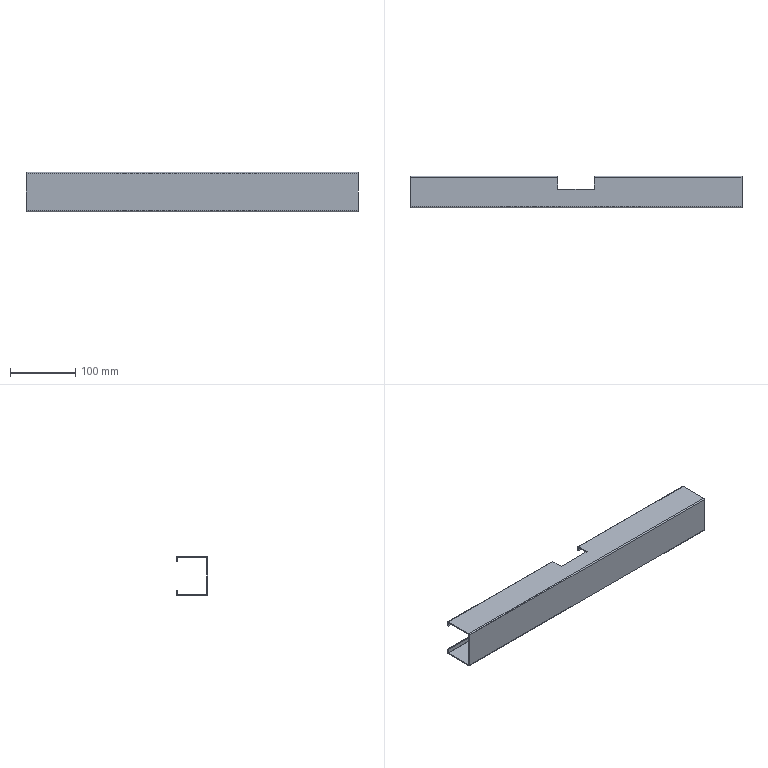Part | 1 solid | 62 faces | box 510 x 48 x 60 mm | volume 121359 mm3 | plane 50 | cylinder 12 | commonest cylinder face diameters 0.4 x6 3.4 x6
STEP:
#1=CARTESIAN_POINT('',(-28.,48.,28.3));
#2=VERTEX_POINT('',#1);
#3=CARTESIAN_POINT('',(-28.,48.,22.));
#4=VERTEX_POINT('',#3);
#5=CARTESIAN_POINT('',(-28.,48.,22.));
#6=DIRECTION('',(0.,0.,-1.));
#7=VECTOR('',#6,1000.);
#8=LINE('',#5,#7);
#9=EDGE_CURVE('',#2,#4,#8,.T.);
#10=ORIENTED_EDGE('',*,*,#9,.F.);
#11=CARTESIAN_POINT('',(-28.,46.5,28.3));
#12=VERTEX_POINT('',#11);
#13=CARTESIAN_POINT('',(-28.,48.,28.3));
#14=DIRECTION('',(0.,-1.,0.));
#15=VECTOR('',#14,1000.);
#16=LINE('',#13,#15);
#17=EDGE_CURVE('',#2,#12,#16,.T.);
#18=ORIENTED_EDGE('',*,*,#17,.T.);
#19=CARTESIAN_POINT('',(-28.,46.5,22.));
#20=VERTEX_POINT('',#19);
#21=CARTESIAN_POINT('',(-28.,46.5,22.));
#22=DIRECTION('',(0.,0.,-1.));
#23=VECTOR('',#22,1000.);
#24=LINE('',#21,#23);
#25=EDGE_CURVE('',#12,#20,#24,.T.);
#26=ORIENTED_EDGE('',*,*,#25,.T.);
#27=CARTESIAN_POINT('',(-28.,48.,22.));
#28=DIRECTION('',(0.,1.,0.));
#29=VECTOR('',#28,1000.);
#30=LINE('',#27,#29);
#31=EDGE_CURVE('',#20,#4,#30,.T.);
#32=ORIENTED_EDGE('',*,*,#31,.T.);
#33=EDGE_LOOP('',(#10,#18,#26,#32));
#34=FACE_OUTER_BOUND('',#33,.T.);
#35=CARTESIAN_POINT('',(-28.,68.,-30.));
#36=DIRECTION('',(-1.,0.,0.));
#37=DIRECTION('',(0.,0.,1.));
#38=AXIS2_PLACEMENT_3D('',#35,#36,#37);
#39=PLANE('',#38);
#40=ADVANCED_FACE('',(#34),#39,.F.);
#41=CARTESIAN_POINT('',(-28.,28.,28.5));
#42=VERTEX_POINT('',#41);
#43=CARTESIAN_POINT('',(-28.,46.3,28.5));
#44=VERTEX_POINT('',#43);
#45=CARTESIAN_POINT('',(-28.,48.,28.5));
#46=DIRECTION('',(0.,1.,0.));
#47=VECTOR('',#46,1000.);
#48=LINE('',#45,#47);
#49=EDGE_CURVE('',#42,#44,#48,.T.);
#50=ORIENTED_EDGE('',*,*,#49,.T.);
#51=CARTESIAN_POINT('',(-28.,46.3,30.));
#52=VERTEX_POINT('',#51);
#53=CARTESIAN_POINT('',(-28.,46.3,28.5));
#54=DIRECTION('',(0.,0.,1.));
#55=VECTOR('',#54,1000.);
#56=LINE('',#53,#55);
#57=EDGE_CURVE('',#44,#52,#56,.T.);
#58=ORIENTED_EDGE('',*,*,#57,.T.);
#59=CARTESIAN_POINT('',(-28.,28.,30.));
#60=VERTEX_POINT('',#59);
#61=CARTESIAN_POINT('',(-28.,48.,30.));
#62=DIRECTION('',(0.,1.,0.));
#63=VECTOR('',#62,1000.);
#64=LINE('',#61,#63);
#65=EDGE_CURVE('',#60,#52,#64,.T.);
#66=ORIENTED_EDGE('',*,*,#65,.F.);
#67=CARTESIAN_POINT('',(-28.,28.,-30.));
#68=DIRECTION('',(0.,0.,1.));
#69=VECTOR('',#68,1000.);
#70=LINE('',#67,#69);
#71=EDGE_CURVE('',#42,#60,#70,.T.);
#72=ORIENTED_EDGE('',*,*,#71,.F.);
#73=EDGE_LOOP('',(#50,#58,#66,#72));
#74=FACE_OUTER_BOUND('',#73,.T.);
#75=CARTESIAN_POINT('',(-28.,68.,-30.));
#76=DIRECTION('',(-1.,0.,0.));
#77=DIRECTION('',(0.,0.,1.));
#78=AXIS2_PLACEMENT_3D('',#75,#76,#77);
#79=PLANE('',#78);
#80=ADVANCED_FACE('',(#74),#79,.F.);
#81=CARTESIAN_POINT('',(28.,46.5,22.));
#82=VERTEX_POINT('',#81);
#83=CARTESIAN_POINT('',(28.,46.5,28.3));
#84=VERTEX_POINT('',#83);
#85=CARTESIAN_POINT('',(28.,46.5,22.));
#86=DIRECTION('',(0.,0.,1.));
#87=VECTOR('',#86,1000.);
#88=LINE('',#85,#87);
#89=EDGE_CURVE('',#82,#84,#88,.T.);
#90=ORIENTED_EDGE('',*,*,#89,.T.);
#91=CARTESIAN_POINT('',(28.,48.,28.3));
#92=VERTEX_POINT('',#91);
#93=CARTESIAN_POINT('',(28.,46.5,28.3));
#94=DIRECTION('',(0.,1.,0.));
#95=VECTOR('',#94,1000.);
#96=LINE('',#93,#95);
#97=EDGE_CURVE('',#84,#92,#96,.T.);
#98=ORIENTED_EDGE('',*,*,#97,.T.);
#99=CARTESIAN_POINT('',(28.,48.,22.));
#100=VERTEX_POINT('',#99);
#101=CARTESIAN_POINT('',(28.,48.,22.));
#102=DIRECTION('',(0.,0.,1.));
#103=VECTOR('',#102,1000.);
#104=LINE('',#101,#103);
#105=EDGE_CURVE('',#100,#92,#104,.T.);
#106=ORIENTED_EDGE('',*,*,#105,.F.);
#107=CARTESIAN_POINT('',(28.,48.,22.));
#108=DIRECTION('',(0.,-1.,0.));
#109=VECTOR('',#108,1000.);
#110=LINE('',#107,#109);
#111=EDGE_CURVE('',#100,#82,#110,.T.);
#112=ORIENTED_EDGE('',*,*,#111,.T.);
#113=EDGE_LOOP('',(#90,#98,#106,#112));
#114=FACE_OUTER_BOUND('',#113,.T.);
#115=CARTESIAN_POINT('',(28.,68.,-30.));
#116=DIRECTION('',(1.,0.,0.));
#117=DIRECTION('',(0.,0.,-1.));
#118=AXIS2_PLACEMENT_3D('',#115,#116,#117);
#119=PLANE('',#118);
#120=ADVANCED_FACE('',(#114),#119,.F.);
#121=CARTESIAN_POINT('',(28.,46.3,30.));
#122=VERTEX_POINT('',#121);
#123=CARTESIAN_POINT('',(28.,28.,30.));
#124=VERTEX_POINT('',#123);
#125=CARTESIAN_POINT('',(28.,48.,30.));
#126=DIRECTION('',(0.,-1.,0.));
#127=VECTOR('',#126,1000.);
#128=LINE('',#125,#127);
#129=EDGE_CURVE('',#122,#124,#128,.T.);
#130=ORIENTED_EDGE('',*,*,#129,.F.);
#131=CARTESIAN_POINT('',(28.,46.3,28.5));
#132=VERTEX_POINT('',#131);
#133=CARTESIAN_POINT('',(28.,46.3,30.));
#134=DIRECTION('',(0.,0.,-1.));
#135=VECTOR('',#134,1000.);
#136=LINE('',#133,#135);
#137=EDGE_CURVE('',#122,#132,#136,.T.);
#138=ORIENTED_EDGE('',*,*,#137,.T.);
#139=CARTESIAN_POINT('',(28.,28.,28.5));
#140=VERTEX_POINT('',#139);
#141=CARTESIAN_POINT('',(28.,48.,28.5));
#142=DIRECTION('',(0.,-1.,0.));
#143=VECTOR('',#142,1000.);
#144=LINE('',#141,#143);
#145=EDGE_CURVE('',#132,#140,#144,.T.);
#146=ORIENTED_EDGE('',*,*,#145,.T.);
#147=CARTESIAN_POINT('',(28.,28.,-30.));
#148=DIRECTION('',(0.,0.,1.));
#149=VECTOR('',#148,1000.);
#150=LINE('',#147,#149);
#151=EDGE_CURVE('',#140,#124,#150,.T.);
#152=ORIENTED_EDGE('',*,*,#151,.T.);
#153=EDGE_LOOP('',(#130,#138,#146,#152));
#154=FACE_OUTER_BOUND('',#153,.T.);
#155=CARTESIAN_POINT('',(28.,68.,-30.));
#156=DIRECTION('',(1.,0.,0.));
#157=DIRECTION('',(0.,0.,-1.));
#158=AXIS2_PLACEMENT_3D('',#155,#156,#157);
#159=PLANE('',#158);
#160=ADVANCED_FACE('',(#154),#159,.F.);
#161=CARTESIAN_POINT('',(-28.,46.5,-22.));
#162=VERTEX_POINT('',#161);
#163=CARTESIAN_POINT('',(-28.,46.5,-28.3));
#164=VERTEX_POINT('',#163);
#165=CARTESIAN_POINT('',(-28.,46.5,-30.));
#166=DIRECTION('',(0.,0.,-1.));
#167=VECTOR('',#166,1000.);
#168=LINE('',#165,#167);
#169=EDGE_CURVE('',#162,#164,#168,.T.);
#170=ORIENTED_EDGE('',*,*,#169,.T.);
#171=CARTESIAN_POINT('',(-28.,48.,-28.3));
#172=VERTEX_POINT('',#171);
#173=CARTESIAN_POINT('',(-28.,46.5,-28.3));
#174=DIRECTION('',(0.,1.,0.));
#175=VECTOR('',#174,1000.);
#176=LINE('',#173,#175);
#177=EDGE_CURVE('',#164,#172,#176,.T.);
#178=ORIENTED_EDGE('',*,*,#177,.T.);
#179=CARTESIAN_POINT('',(-28.,48.,-22.));
#180=VERTEX_POINT('',#179);
#181=CARTESIAN_POINT('',(-28.,48.,-30.));
#182=DIRECTION('',(0.,0.,-1.));
#183=VECTOR('',#182,1000.);
#184=LINE('',#181,#183);
#185=EDGE_CURVE('',#180,#172,#184,.T.);
#186=ORIENTED_EDGE('',*,*,#185,.F.);
#187=CARTESIAN_POINT('',(-28.,46.5,-22.));
#188=DIRECTION('',(0.,-1.,0.));
#189=VECTOR('',#188,1000.);
#190=LINE('',#187,#189);
#191=EDGE_CURVE('',#180,#162,#190,.T.);
#192=ORIENTED_EDGE('',*,*,#191,.T.);
#193=EDGE_LOOP('',(#170,#178,#186,#192));
#194=FACE_OUTER_BOUND('',#193,.T.);
#195=CARTESIAN_POINT('',(-28.,68.,-30.));
#196=DIRECTION('',(-1.,0.,0.));
#197=DIRECTION('',(0.,0.,1.));
#198=AXIS2_PLACEMENT_3D('',#195,#196,#197);
#199=PLANE('',#198);
#200=ADVANCED_FACE('',(#194),#199,.F.);
#201=CARTESIAN_POINT('',(-28.,46.3,-30.));
#202=VERTEX_POINT('',#201);
#203=CARTESIAN_POINT('',(-28.,28.,-30.));
#204=VERTEX_POINT('',#203);
#205=CARTESIAN_POINT('',(-28.,68.,-30.));
#206=DIRECTION('',(0.,-1.,0.));
#207=VECTOR('',#206,1000.);
#208=LINE('',#205,#207);
#209=EDGE_CURVE('',#202,#204,#208,.T.);
#210=ORIENTED_EDGE('',*,*,#209,.F.);
#211=CARTESIAN_POINT('',(-28.,46.3,-28.5));
#212=VERTEX_POINT('',#211);
#213=CARTESIAN_POINT('',(-28.,46.3,-30.));
#214=DIRECTION('',(0.,0.,1.));
#215=VECTOR('',#214,1000.);
#216=LINE('',#213,#215);
#217=EDGE_CURVE('',#202,#212,#216,.T.);
#218=ORIENTED_EDGE('',*,*,#217,.T.);
#219=CARTESIAN_POINT('',(-28.,28.,-28.5));
#220=VERTEX_POINT('',#219);
#221=CARTESIAN_POINT('',(-28.,0.,-28.5));
#222=DIRECTION('',(0.,-1.,0.));
#223=VECTOR('',#222,1000.);
#224=LINE('',#221,#223);
#225=EDGE_CURVE('',#212,#220,#224,.T.);
#226=ORIENTED_EDGE('',*,*,#225,.T.);
#227=CARTESIAN_POINT('',(-28.,28.,-30.));
#228=DIRECTION('',(0.,0.,1.));
#229=VECTOR('',#228,1000.);
#230=LINE('',#227,#229);
#231=EDGE_CURVE('',#204,#220,#230,.T.);
#232=ORIENTED_EDGE('',*,*,#231,.F.);
#233=EDGE_LOOP('',(#210,#218,#226,#232));
#234=FACE_OUTER_BOUND('',#233,.T.);
#235=CARTESIAN_POINT('',(-28.,68.,-30.));
#236=DIRECTION('',(-1.,0.,0.));
#237=DIRECTION('',(0.,0.,1.));
#238=AXIS2_PLACEMENT_3D('',#235,#236,#237);
#239=PLANE('',#238);
#240=ADVANCED_FACE('',(#234),#239,.F.);
#241=CARTESIAN_POINT('',(28.,48.,-28.3));
#242=VERTEX_POINT('',#241);
#243=CARTESIAN_POINT('',(28.,48.,-22.));
#244=VERTEX_POINT('',#243);
#245=CARTESIAN_POINT('',(28.,48.,-30.));
#246=DIRECTION('',(0.,0.,1.));
#247=VECTOR('',#246,1000.);
#248=LINE('',#245,#247);
#249=EDGE_CURVE('',#242,#244,#248,.T.);
#250=ORIENTED_EDGE('',*,*,#249,.F.);
#251=CARTESIAN_POINT('',(28.,46.5,-28.3));
#252=VERTEX_POINT('',#251);
#253=CARTESIAN_POINT('',(28.,48.,-28.3));
#254=DIRECTION('',(0.,-1.,0.));
#255=VECTOR('',#254,1000.);
#256=LINE('',#253,#255);
#257=EDGE_CURVE('',#242,#252,#256,.T.);
#258=ORIENTED_EDGE('',*,*,#257,.T.);
#259=CARTESIAN_POINT('',(28.,46.5,-22.));
#260=VERTEX_POINT('',#259);
#261=CARTESIAN_POINT('',(28.,46.5,-30.));
#262=DIRECTION('',(0.,0.,1.));
#263=VECTOR('',#262,1000.);
#264=LINE('',#261,#263);
#265=EDGE_CURVE('',#252,#260,#264,.T.);
#266=ORIENTED_EDGE('',*,*,#265,.T.);
#267=CARTESIAN_POINT('',(28.,46.5,-22.));
#268=DIRECTION('',(0.,1.,0.));
#269=VECTOR('',#268,1000.);
#270=LINE('',#267,#269);
#271=EDGE_CURVE('',#260,#244,#270,.T.);
#272=ORIENTED_EDGE('',*,*,#271,.T.);
#273=EDGE_LOOP('',(#250,#258,#266,#272));
#274=FACE_OUTER_BOUND('',#273,.T.);
#275=CARTESIAN_POINT('',(28.,68.,-30.));
#276=DIRECTION('',(1.,0.,0.));
#277=DIRECTION('',(0.,0.,-1.));
#278=AXIS2_PLACEMENT_3D('',#275,#276,#277);
#279=PLANE('',#278);
#280=ADVANCED_FACE('',(#274),#279,.F.);
#281=CARTESIAN_POINT('',(28.,28.,-28.5));
#282=VERTEX_POINT('',#281);
#283=CARTESIAN_POINT('',(28.,46.3,-28.5));
#284=VERTEX_POINT('',#283);
#285=CARTESIAN_POINT('',(28.,0.,-28.5));
#286=DIRECTION('',(0.,1.,0.));
#287=VECTOR('',#286,1000.);
#288=LINE('',#285,#287);
#289=EDGE_CURVE('',#282,#284,#288,.T.);
#290=ORIENTED_EDGE('',*,*,#289,.T.);
#291=CARTESIAN_POINT('',(28.,46.3,-30.));
#292=VERTEX_POINT('',#291);
#293=CARTESIAN_POINT('',(28.,46.3,-28.5));
#294=DIRECTION('',(0.,0.,-1.));
#295=VECTOR('',#294,1000.);
#296=LINE('',#293,#295);
#297=EDGE_CURVE('',#284,#292,#296,.T.);
#298=ORIENTED_EDGE('',*,*,#297,.T.);
#299=CARTESIAN_POINT('',(28.,28.,-30.));
#300=VERTEX_POINT('',#299);
#301=CARTESIAN_POINT('',(28.,68.,-30.));
#302=DIRECTION('',(0.,1.,0.));
#303=VECTOR('',#302,1000.);
#304=LINE('',#301,#303);
#305=EDGE_CURVE('',#300,#292,#304,.T.);
#306=ORIENTED_EDGE('',*,*,#305,.F.);
#307=CARTESIAN_POINT('',(28.,28.,-30.));
#308=DIRECTION('',(0.,0.,1.));
#309=VECTOR('',#308,1000.);
#310=LINE('',#307,#309);
#311=EDGE_CURVE('',#300,#282,#310,.T.);
#312=ORIENTED_EDGE('',*,*,#311,.T.);
#313=EDGE_LOOP('',(#290,#298,#306,#312));
#314=FACE_OUTER_BOUND('',#313,.T.);
#315=CARTESIAN_POINT('',(28.,68.,-30.));
#316=DIRECTION('',(1.,0.,0.));
#317=DIRECTION('',(0.,0.,-1.));
#318=AXIS2_PLACEMENT_3D('',#315,#316,#317);
#319=PLANE('',#318);
#320=ADVANCED_FACE('',(#314),#319,.F.);
#321=CARTESIAN_POINT('',(255.,48.,-28.3));
#322=VERTEX_POINT('',#321);
#323=CARTESIAN_POINT('',(255.,48.,-28.3));
#324=DIRECTION('',(-1.,0.,0.));
#325=VECTOR('',#324,1000.);
#326=LINE('',#323,#325);
#327=EDGE_CURVE('',#322,#242,#326,.T.);
#328=ORIENTED_EDGE('',*,*,#327,.T.);
#329=ORIENTED_EDGE('',*,*,#249,.T.);
#330=CARTESIAN_POINT('',(255.,48.,-22.));
#331=VERTEX_POINT('',#330);
#332=CARTESIAN_POINT('',(255.,48.,-22.));
#333=DIRECTION('',(-1.,0.,0.));
#334=VECTOR('',#333,1000.);
#335=LINE('',#332,#334);
#336=EDGE_CURVE('',#331,#244,#335,.T.);
#337=ORIENTED_EDGE('',*,*,#336,.F.);
#338=CARTESIAN_POINT('',(255.,48.,-30.));
#339=DIRECTION('',(0.,0.,1.));
#340=VECTOR('',#339,1000.);
#341=LINE('',#338,#340);
#342=EDGE_CURVE('',#322,#331,#341,.T.);
#343=ORIENTED_EDGE('',*,*,#342,.F.);
#344=EDGE_LOOP('',(#328,#329,#337,#343));
#345=FACE_OUTER_BOUND('',#344,.T.);
#346=CARTESIAN_POINT('',(255.,48.,-30.));
#347=DIRECTION('',(0.,-1.,0.));
#348=DIRECTION('',(0.,0.,-1.));
#349=AXIS2_PLACEMENT_3D('',#346,#347,#348);
#350=PLANE('',#349);
#351=ADVANCED_FACE('',(#345),#350,.F.);
#352=ORIENTED_EDGE('',*,*,#271,.F.);
#353=CARTESIAN_POINT('',(255.,46.5,-22.));
#354=VERTEX_POINT('',#353);
#355=CARTESIAN_POINT('',(255.,46.5,-22.));
#356=DIRECTION('',(-1.,0.,0.));
#357=VECTOR('',#356,1000.);
#358=LINE('',#355,#357);
#359=EDGE_CURVE('',#354,#260,#358,.T.);
#360=ORIENTED_EDGE('',*,*,#359,.F.);
#361=CARTESIAN_POINT('',(255.,46.5,-22.));
#362=DIRECTION('',(0.,1.,0.));
#363=VECTOR('',#362,1000.);
#364=LINE('',#361,#363);
#365=EDGE_CURVE('',#354,#331,#364,.T.);
#366=ORIENTED_EDGE('',*,*,#365,.T.);
#367=ORIENTED_EDGE('',*,*,#336,.T.);
#368=EDGE_LOOP('',(#352,#360,#366,#367));
#369=FACE_OUTER_BOUND('',#368,.T.);
#370=CARTESIAN_POINT('',(255.,46.5,-22.));
#371=DIRECTION('',(0.,0.,1.));
#372=DIRECTION('',(1.,0.,0.));
#373=AXIS2_PLACEMENT_3D('',#370,#371,#372);
#374=PLANE('',#373);
#375=ADVANCED_FACE('',(#369),#374,.T.);
#376=ORIENTED_EDGE('',*,*,#265,.F.);
#377=CARTESIAN_POINT('',(255.,46.5,-28.3));
#378=VERTEX_POINT('',#377);
#379=CARTESIAN_POINT('',(255.,46.5,-28.3));
#380=DIRECTION('',(-1.,0.,0.));
#381=VECTOR('',#380,1000.);
#382=LINE('',#379,#381);
#383=EDGE_CURVE('',#378,#252,#382,.T.);
#384=ORIENTED_EDGE('',*,*,#383,.F.);
#385=CARTESIAN_POINT('',(255.,46.5,-30.));
#386=DIRECTION('',(0.,0.,1.));
#387=VECTOR('',#386,1000.);
#388=LINE('',#385,#387);
#389=EDGE_CURVE('',#378,#354,#388,.T.);
#390=ORIENTED_EDGE('',*,*,#389,.T.);
#391=ORIENTED_EDGE('',*,*,#359,.T.);
#392=EDGE_LOOP('',(#376,#384,#390,#391));
#393=FACE_OUTER_BOUND('',#392,.T.);
#394=CARTESIAN_POINT('',(255.,46.5,-30.));
#395=DIRECTION('',(0.,-1.,0.));
#396=DIRECTION('',(0.,0.,-1.));
#397=AXIS2_PLACEMENT_3D('',#394,#395,#396);
#398=PLANE('',#397);
#399=ADVANCED_FACE('',(#393),#398,.T.);
#400=CARTESIAN_POINT('',(28.,46.3,-28.3));
#401=DIRECTION('',(1.,0.,0.));
#402=DIRECTION('',(0.,0.,-1.));
#403=AXIS2_PLACEMENT_3D('',#400,#401,#402);
#404=CIRCLE('',#403,0.2);
#405=EDGE_CURVE('',#284,#252,#404,.T.);
#406=ORIENTED_EDGE('',*,*,#405,.F.);
#407=CARTESIAN_POINT('',(255.,46.3,-28.5));
#408=VERTEX_POINT('',#407);
#409=CARTESIAN_POINT('',(255.,46.3,-28.5));
#410=DIRECTION('',(-1.,0.,0.));
#411=VECTOR('',#410,1000.);
#412=LINE('',#409,#411);
#413=EDGE_CURVE('',#408,#284,#412,.T.);
#414=ORIENTED_EDGE('',*,*,#413,.F.);
#415=CARTESIAN_POINT('',(255.,46.3,-28.3));
#416=DIRECTION('',(1.,0.,0.));
#417=DIRECTION('',(0.,0.,-1.));
#418=AXIS2_PLACEMENT_3D('',#415,#416,#417);
#419=CIRCLE('',#418,0.2);
#420=EDGE_CURVE('',#408,#378,#419,.T.);
#421=ORIENTED_EDGE('',*,*,#420,.T.);
#422=ORIENTED_EDGE('',*,*,#383,.T.);
#423=EDGE_LOOP('',(#406,#414,#421,#422));
#424=FACE_OUTER_BOUND('',#423,.T.);
#425=CARTESIAN_POINT('',(255.,46.3,-28.3));
#426=DIRECTION('',(-1.,0.,0.));
#427=DIRECTION('',(0.,0.,1.));
#428=AXIS2_PLACEMENT_3D('',#425,#426,#427);
#429=CYLINDRICAL_SURFACE('',#428,0.2);
#430=ADVANCED_FACE('',(#424),#429,.F.);
#431=CARTESIAN_POINT('',(28.,46.3,28.3));
#432=DIRECTION('',(1.,0.,0.));
#433=DIRECTION('',(0.,0.,-1.));
#434=AXIS2_PLACEMENT_3D('',#431,#432,#433);
#435=CIRCLE('',#434,0.2);
#436=EDGE_CURVE('',#84,#132,#435,.T.);
#437=ORIENTED_EDGE('',*,*,#436,.F.);
#438=CARTESIAN_POINT('',(255.,46.5,28.3));
#439=VERTEX_POINT('',#438);
#440=CARTESIAN_POINT('',(255.,46.5,28.3));
#441=DIRECTION('',(-1.,0.,0.));
#442=VECTOR('',#441,1000.);
#443=LINE('',#440,#442);
#444=EDGE_CURVE('',#439,#84,#443,.T.);
#445=ORIENTED_EDGE('',*,*,#444,.F.);
#446=CARTESIAN_POINT('',(255.,46.3,28.5));
#447=VERTEX_POINT('',#446);
#448=CARTESIAN_POINT('',(255.,46.3,28.3));
#449=DIRECTION('',(1.,0.,0.));
#450=DIRECTION('',(0.,0.,-1.));
#451=AXIS2_PLACEMENT_3D('',#448,#449,#450);
#452=CIRCLE('',#451,0.2);
#453=EDGE_CURVE('',#439,#447,#452,.T.);
#454=ORIENTED_EDGE('',*,*,#453,.T.);
#455=CARTESIAN_POINT('',(255.,46.3,28.5));
#456=DIRECTION('',(-1.,0.,0.));
#457=VECTOR('',#456,1000.);
#458=LINE('',#455,#457);
#459=EDGE_CURVE('',#447,#132,#458,.T.);
#460=ORIENTED_EDGE('',*,*,#459,.T.);
#461=EDGE_LOOP('',(#437,#445,#454,#460));
#462=FACE_OUTER_BOUND('',#461,.T.);
#463=CARTESIAN_POINT('',(255.,46.3,28.3));
#464=DIRECTION('',(-1.,0.,0.));
#465=DIRECTION('',(0.,0.,1.));
#466=AXIS2_PLACEMENT_3D('',#463,#464,#465);
#467=CYLINDRICAL_SURFACE('',#466,0.2);
#468=ADVANCED_FACE('',(#462),#467,.F.);
#469=ORIENTED_EDGE('',*,*,#89,.F.);
#470=CARTESIAN_POINT('',(255.,46.5,22.));
#471=VERTEX_POINT('',#470);
#472=CARTESIAN_POINT('',(255.,46.5,22.));
#473=DIRECTION('',(-1.,0.,0.));
#474=VECTOR('',#473,1000.);
#475=LINE('',#472,#474);
#476=EDGE_CURVE('',#471,#82,#475,.T.);
#477=ORIENTED_EDGE('',*,*,#476,.F.);
#478=CARTESIAN_POINT('',(255.,46.5,22.));
#479=DIRECTION('',(0.,0.,1.));
#480=VECTOR('',#479,1000.);
#481=LINE('',#478,#480);
#482=EDGE_CURVE('',#471,#439,#481,.T.);
#483=ORIENTED_EDGE('',*,*,#482,.T.);
#484=ORIENTED_EDGE('',*,*,#444,.T.);
#485=EDGE_LOOP('',(#469,#477,#483,#484));
#486=FACE_OUTER_BOUND('',#485,.T.);
#487=CARTESIAN_POINT('',(255.,46.5,22.));
#488=DIRECTION('',(0.,-1.,0.));
#489=DIRECTION('',(0.,0.,-1.));
#490=AXIS2_PLACEMENT_3D('',#487,#488,#489);
#491=PLANE('',#490);
#492=ADVANCED_FACE('',(#486),#491,.T.);
#493=ORIENTED_EDGE('',*,*,#111,.F.);
#494=CARTESIAN_POINT('',(255.,48.,22.));
#495=VERTEX_POINT('',#494);
#496=CARTESIAN_POINT('',(255.,48.,22.));
#497=DIRECTION('',(-1.,0.,0.));
#498=VECTOR('',#497,1000.);
#499=LINE('',#496,#498);
#500=EDGE_CURVE('',#495,#100,#499,.T.);
#501=ORIENTED_EDGE('',*,*,#500,.F.);
#502=CARTESIAN_POINT('',(255.,48.,22.));
#503=DIRECTION('',(0.,-1.,0.));
#504=VECTOR('',#503,1000.);
#505=LINE('',#502,#504);
#506=EDGE_CURVE('',#495,#471,#505,.T.);
#507=ORIENTED_EDGE('',*,*,#506,.T.);
#508=ORIENTED_EDGE('',*,*,#476,.T.);
#509=EDGE_LOOP('',(#493,#501,#507,#508));
#510=FACE_OUTER_BOUND('',#509,.T.);
#511=CARTESIAN_POINT('',(255.,48.,22.));
#512=DIRECTION('',(0.,0.,-1.));
#513=DIRECTION('',(-1.,0.,0.));
#514=AXIS2_PLACEMENT_3D('',#511,#512,#513);
#515=PLANE('',#514);
#516=ADVANCED_FACE('',(#510),#515,.T.);
#517=ORIENTED_EDGE('',*,*,#500,.T.);
#518=ORIENTED_EDGE('',*,*,#105,.T.);
#519=CARTESIAN_POINT('',(255.,48.,28.3));
#520=VERTEX_POINT('',#519);
#521=CARTESIAN_POINT('',(255.,48.,28.3));
#522=DIRECTION('',(-1.,0.,0.));
#523=VECTOR('',#522,1000.);
#524=LINE('',#521,#523);
#525=EDGE_CURVE('',#520,#92,#524,.T.);
#526=ORIENTED_EDGE('',*,*,#525,.F.);
#527=CARTESIAN_POINT('',(255.,48.,22.));
#528=DIRECTION('',(0.,0.,1.));
#529=VECTOR('',#528,1000.);
#530=LINE('',#527,#529);
#531=EDGE_CURVE('',#495,#520,#530,.T.);
#532=ORIENTED_EDGE('',*,*,#531,.F.);
#533=EDGE_LOOP('',(#517,#518,#526,#532));
#534=FACE_OUTER_BOUND('',#533,.T.);
#535=CARTESIAN_POINT('',(255.,48.,22.));
#536=DIRECTION('',(0.,-1.,0.));
#537=DIRECTION('',(0.,0.,-1.));
#538=AXIS2_PLACEMENT_3D('',#535,#536,#537);
#539=PLANE('',#538);
#540=ADVANCED_FACE('',(#534),#539,.F.);
#541=ORIENTED_EDGE('',*,*,#525,.T.);
#542=CARTESIAN_POINT('',(28.,46.3,28.3));
#543=DIRECTION('',(1.,0.,0.));
#544=DIRECTION('',(0.,0.,-1.));
#545=AXIS2_PLACEMENT_3D('',#542,#543,#544);
#546=CIRCLE('',#545,1.7);
#547=EDGE_CURVE('',#92,#122,#546,.T.);
#548=ORIENTED_EDGE('',*,*,#547,.T.);
#549=CARTESIAN_POINT('',(255.,46.3,30.));
#550=VERTEX_POINT('',#549);
#551=CARTESIAN_POINT('',(255.,46.3,30.));
#552=DIRECTION('',(-1.,0.,0.));
#553=VECTOR('',#552,1000.);
#554=LINE('',#551,#553);
#555=EDGE_CURVE('',#550,#122,#554,.T.);
#556=ORIENTED_EDGE('',*,*,#555,.F.);
#557=CARTESIAN_POINT('',(255.,46.3,28.3));
#558=DIRECTION('',(1.,0.,0.));
#559=DIRECTION('',(0.,0.,1.));
#560=AXIS2_PLACEMENT_3D('',#557,#558,#559);
#561=CIRCLE('',#560,1.7);
#562=EDGE_CURVE('',#520,#550,#561,.T.);
#563=ORIENTED_EDGE('',*,*,#562,.F.);
#564=EDGE_LOOP('',(#541,#548,#556,#563));
#565=FACE_OUTER_BOUND('',#564,.T.);
#566=CARTESIAN_POINT('',(255.,46.3,28.3));
#567=DIRECTION('',(-1.,0.,0.));
#568=DIRECTION('',(0.,0.,1.));
#569=AXIS2_PLACEMENT_3D('',#566,#567,#568);
#570=CYLINDRICAL_SURFACE('',#569,1.7);
#571=ADVANCED_FACE('',(#565),#570,.T.);
#572=CARTESIAN_POINT('',(255.,46.3,-30.));
#573=VERTEX_POINT('',#572);
#574=CARTESIAN_POINT('',(255.,46.3,-30.));
#575=DIRECTION('',(-1.,0.,0.));
#576=VECTOR('',#575,1000.);
#577=LINE('',#574,#576);
#578=EDGE_CURVE('',#573,#292,#577,.T.);
#579=ORIENTED_EDGE('',*,*,#578,.T.);
#580=CARTESIAN_POINT('',(28.,46.3,-28.3));
#581=DIRECTION('',(1.,0.,0.));
#582=DIRECTION('',(0.,0.,-1.));
#583=AXIS2_PLACEMENT_3D('',#580,#581,#582);
#584=CIRCLE('',#583,1.7);
#585=EDGE_CURVE('',#292,#242,#584,.T.);
#586=ORIENTED_EDGE('',*,*,#585,.T.);
#587=ORIENTED_EDGE('',*,*,#327,.F.);
#588=CARTESIAN_POINT('',(255.,46.3,-28.3));
#589=DIRECTION('',(1.,0.,0.));
#590=DIRECTION('',(0.,0.,1.));
#591=AXIS2_PLACEMENT_3D('',#588,#589,#590);
#592=CIRCLE('',#591,1.7);
#593=EDGE_CURVE('',#573,#322,#592,.T.);
#594=ORIENTED_EDGE('',*,*,#593,.F.);
#595=EDGE_LOOP('',(#579,#586,#587,#594));
#596=FACE_OUTER_BOUND('',#595,.T.);
#597=CARTESIAN_POINT('',(255.,46.3,-28.3));
#598=DIRECTION('',(-1.,0.,0.));
#599=DIRECTION('',(0.,0.,1.));
#600=AXIS2_PLACEMENT_3D('',#597,#598,#599);
#601=CYLINDRICAL_SURFACE('',#600,1.7);
#602=ADVANCED_FACE('',(#596),#601,.T.);
#603=CARTESIAN_POINT('',(255.,48.,28.3));
#604=DIRECTION('',(0.,-1.,0.));
#605=VECTOR('',#604,1000.);
#606=LINE('',#603,#605);
#607=EDGE_CURVE('',#520,#439,#606,.T.);
#608=ORIENTED_EDGE('',*,*,#607,.F.);
#609=ORIENTED_EDGE('',*,*,#562,.T.);
#610=CARTESIAN_POINT('',(255.,46.3,28.5));
#611=DIRECTION('',(0.,0.,1.));
#612=VECTOR('',#611,1000.);
#613=LINE('',#610,#612);
#614=EDGE_CURVE('',#447,#550,#613,.T.);
#615=ORIENTED_EDGE('',*,*,#614,.F.);
#616=ORIENTED_EDGE('',*,*,#453,.F.);
#617=EDGE_LOOP('',(#608,#609,#615,#616));
#618=FACE_OUTER_BOUND('',#617,.T.);
#619=CARTESIAN_POINT('',(255.,48.,28.3));
#620=DIRECTION('',(1.,0.,0.));
#621=DIRECTION('',(0.,0.,-1.));
#622=AXIS2_PLACEMENT_3D('',#619,#620,#621);
#623=PLANE('',#622);
#624=ADVANCED_FACE('',(#618),#623,.T.);
#625=ORIENTED_EDGE('',*,*,#531,.T.);
#626=ORIENTED_EDGE('',*,*,#607,.T.);
#627=ORIENTED_EDGE('',*,*,#482,.F.);
#628=ORIENTED_EDGE('',*,*,#506,.F.);
#629=EDGE_LOOP('',(#625,#626,#627,#628));
#630=FACE_OUTER_BOUND('',#629,.T.);
#631=CARTESIAN_POINT('',(255.,46.3,28.5));
#632=DIRECTION('',(1.,0.,0.));
#633=DIRECTION('',(0.,0.,-1.));
#634=AXIS2_PLACEMENT_3D('',#631,#632,#633);
#635=PLANE('',#634);
#636=ADVANCED_FACE('',(#630),#635,.T.);
#637=CARTESIAN_POINT('',(-255.,46.3,30.));
#638=VERTEX_POINT('',#637);
#639=CARTESIAN_POINT('',(-255.,46.3,28.5));
#640=VERTEX_POINT('',#639);
#641=CARTESIAN_POINT('',(-255.,46.3,30.));
#642=DIRECTION('',(0.,0.,-1.));
#643=VECTOR('',#642,1000.);
#644=LINE('',#641,#643);
#645=EDGE_CURVE('',#638,#640,#644,.T.);
#646=ORIENTED_EDGE('',*,*,#645,.F.);
#647=CARTESIAN_POINT('',(-255.,48.,28.3));
#648=VERTEX_POINT('',#647);
#649=CARTESIAN_POINT('',(-255.,46.3,28.3));
#650=DIRECTION('',(1.,0.,0.));
#651=DIRECTION('',(0.,0.,1.));
#652=AXIS2_PLACEMENT_3D('',#649,#650,#651);
#653=CIRCLE('',#652,1.7);
#654=EDGE_CURVE('',#648,#638,#653,.T.);
#655=ORIENTED_EDGE('',*,*,#654,.F.);
#656=CARTESIAN_POINT('',(-255.,46.5,28.3));
#657=VERTEX_POINT('',#656);
#658=CARTESIAN_POINT('',(-255.,46.5,28.3));
#659=DIRECTION('',(0.,1.,0.));
#660=VECTOR('',#659,1000.);
#661=LINE('',#658,#660);
#662=EDGE_CURVE('',#657,#648,#661,.T.);
#663=ORIENTED_EDGE('',*,*,#662,.F.);
#664=CARTESIAN_POINT('',(-255.,46.3,28.3));
#665=DIRECTION('',(1.,0.,0.));
#666=DIRECTION('',(0.,0.,-1.));
#667=AXIS2_PLACEMENT_3D('',#664,#665,#666);
#668=CIRCLE('',#667,0.2);
#669=EDGE_CURVE('',#657,#640,#668,.T.);
#670=ORIENTED_EDGE('',*,*,#669,.T.);
#671=EDGE_LOOP('',(#646,#655,#663,#670));
#672=FACE_OUTER_BOUND('',#671,.T.);
#673=CARTESIAN_POINT('',(-255.,46.3,30.));
#674=DIRECTION('',(-1.,0.,0.));
#675=DIRECTION('',(0.,0.,1.));
#676=AXIS2_PLACEMENT_3D('',#673,#674,#675);
#677=PLANE('',#676);
#678=ADVANCED_FACE('',(#672),#677,.T.);
#679=CARTESIAN_POINT('',(-255.,1.7,30.));
#680=VERTEX_POINT('',#679);
#681=CARTESIAN_POINT('',(-255.,48.,30.));
#682=DIRECTION('',(0.,-1.,0.));
#683=VECTOR('',#682,1000.);
#684=LINE('',#681,#683);
#685=EDGE_CURVE('',#638,#680,#684,.T.);
#686=ORIENTED_EDGE('',*,*,#685,.F.);
#687=ORIENTED_EDGE('',*,*,#645,.T.);
#688=CARTESIAN_POINT('',(-255.,1.7,28.5));
#689=VERTEX_POINT('',#688);
#690=CARTESIAN_POINT('',(-255.,48.,28.5));
#691=DIRECTION('',(0.,-1.,0.));
#692=VECTOR('',#691,1000.);
#693=LINE('',#690,#692);
#694=EDGE_CURVE('',#640,#689,#693,.T.);
#695=ORIENTED_EDGE('',*,*,#694,.T.);
#696=CARTESIAN_POINT('',(-255.,1.7,28.5));
#697=DIRECTION('',(0.,0.,1.));
#698=VECTOR('',#697,1000.);
#699=LINE('',#696,#698);
#700=EDGE_CURVE('',#689,#680,#699,.T.);
#701=ORIENTED_EDGE('',*,*,#700,.T.);
#702=EDGE_LOOP('',(#686,#687,#695,#701));
#703=FACE_OUTER_BOUND('',#702,.T.);
#704=CARTESIAN_POINT('',(-255.,46.5,28.3));
#705=DIRECTION('',(-1.,0.,0.));
#706=DIRECTION('',(0.,0.,1.));
#707=AXIS2_PLACEMENT_3D('',#704,#705,#706);
#708=PLANE('',#707);
#709=ADVANCED_FACE('',(#703),#708,.T.);
#710=CARTESIAN_POINT('',(255.,1.7,30.));
#711=VERTEX_POINT('',#710);
#712=CARTESIAN_POINT('',(255.,1.7,28.5));
#713=VERTEX_POINT('',#712);
#714=CARTESIAN_POINT('',(255.,1.7,30.));
#715=DIRECTION('',(0.,0.,-1.));
#716=VECTOR('',#715,1000.);
#717=LINE('',#714,#716);
#718=EDGE_CURVE('',#711,#713,#717,.T.);
#719=ORIENTED_EDGE('',*,*,#718,.F.);
#720=CARTESIAN_POINT('',(255.,0.,28.3));
#721=VERTEX_POINT('',#720);
#722=CARTESIAN_POINT('',(255.,1.7,28.3));
#723=DIRECTION('',(1.,0.,0.));
#724=DIRECTION('',(0.,0.,1.));
#725=AXIS2_PLACEMENT_3D('',#722,#723,#724);
#726=CIRCLE('',#725,1.7);
#727=EDGE_CURVE('',#711,#721,#726,.T.);
#728=ORIENTED_EDGE('',*,*,#727,.T.);
#729=CARTESIAN_POINT('',(255.,1.5,28.3));
#730=VERTEX_POINT('',#729);
#731=CARTESIAN_POINT('',(255.,1.5,28.3));
#732=DIRECTION('',(0.,-1.,0.));
#733=VECTOR('',#732,1000.);
#734=LINE('',#731,#733);
#735=EDGE_CURVE('',#730,#721,#734,.T.);
#736=ORIENTED_EDGE('',*,*,#735,.F.);
#737=CARTESIAN_POINT('',(255.,1.7,28.3));
#738=DIRECTION('',(1.,0.,0.));
#739=DIRECTION('',(0.,0.,-1.));
#740=AXIS2_PLACEMENT_3D('',#737,#738,#739);
#741=CIRCLE('',#740,0.2);
#742=EDGE_CURVE('',#713,#730,#741,.T.);
#743=ORIENTED_EDGE('',*,*,#742,.F.);
#744=EDGE_LOOP('',(#719,#728,#736,#743));
#745=FACE_OUTER_BOUND('',#744,.T.);
#746=CARTESIAN_POINT('',(255.,1.7,30.));
#747=DIRECTION('',(1.,0.,0.));
#748=DIRECTION('',(0.,0.,-1.));
#749=AXIS2_PLACEMENT_3D('',#746,#747,#748);
#750=PLANE('',#749);
#751=ADVANCED_FACE('',(#745),#750,.T.);
#752=CARTESIAN_POINT('',(255.,48.,30.));
#753=DIRECTION('',(0.,-1.,0.));
#754=VECTOR('',#753,1000.);
#755=LINE('',#752,#754);
#756=EDGE_CURVE('',#550,#711,#755,.T.);
#757=ORIENTED_EDGE('',*,*,#756,.T.);
#758=ORIENTED_EDGE('',*,*,#718,.T.);
#759=CARTESIAN_POINT('',(255.,48.,28.5));
#760=DIRECTION('',(0.,-1.,0.));
#761=VECTOR('',#760,1000.);
#762=LINE('',#759,#761);
#763=EDGE_CURVE('',#447,#713,#762,.T.);
#764=ORIENTED_EDGE('',*,*,#763,.F.);
#765=ORIENTED_EDGE('',*,*,#614,.T.);
#766=EDGE_LOOP('',(#757,#758,#764,#765));
#767=FACE_OUTER_BOUND('',#766,.T.);
#768=CARTESIAN_POINT('',(255.,1.5,28.3));
#769=DIRECTION('',(1.,0.,0.));
#770=DIRECTION('',(0.,0.,-1.));
#771=AXIS2_PLACEMENT_3D('',#768,#769,#770);
#772=PLANE('',#771);
#773=ADVANCED_FACE('',(#767),#772,.T.);
#774=CARTESIAN_POINT('',(-255.,0.,28.3));
#775=VERTEX_POINT('',#774);
#776=CARTESIAN_POINT('',(-255.,1.5,28.3));
#777=VERTEX_POINT('',#776);
#778=CARTESIAN_POINT('',(-255.,0.,28.3));
#779=DIRECTION('',(0.,1.,0.));
#780=VECTOR('',#779,1000.);
#781=LINE('',#778,#780);
#782=EDGE_CURVE('',#775,#777,#781,.T.);
#783=ORIENTED_EDGE('',*,*,#782,.F.);
#784=CARTESIAN_POINT('',(-255.,1.7,28.3));
#785=DIRECTION('',(1.,0.,0.));
#786=DIRECTION('',(0.,0.,1.));
#787=AXIS2_PLACEMENT_3D('',#784,#785,#786);
#788=CIRCLE('',#787,1.7);
#789=EDGE_CURVE('',#680,#775,#788,.T.);
#790=ORIENTED_EDGE('',*,*,#789,.F.);
#791=ORIENTED_EDGE('',*,*,#700,.F.);
#792=CARTESIAN_POINT('',(-255.,1.7,28.3));
#793=DIRECTION('',(1.,0.,0.));
#794=DIRECTION('',(0.,0.,-1.));
#795=AXIS2_PLACEMENT_3D('',#792,#793,#794);
#796=CIRCLE('',#795,0.2);
#797=EDGE_CURVE('',#689,#777,#796,.T.);
#798=ORIENTED_EDGE('',*,*,#797,.T.);
#799=EDGE_LOOP('',(#783,#790,#791,#798));
#800=FACE_OUTER_BOUND('',#799,.T.);
#801=CARTESIAN_POINT('',(-255.,0.,28.3));
#802=DIRECTION('',(-1.,0.,0.));
#803=DIRECTION('',(0.,0.,1.));
#804=AXIS2_PLACEMENT_3D('',#801,#802,#803);
#805=PLANE('',#804);
#806=ADVANCED_FACE('',(#800),#805,.T.);
#807=CARTESIAN_POINT('',(-255.,0.,-28.3));
#808=VERTEX_POINT('',#807);
#809=CARTESIAN_POINT('',(-255.,0.,30.));
#810=DIRECTION('',(0.,0.,-1.));
#811=VECTOR('',#810,1000.);
#812=LINE('',#809,#811);
#813=EDGE_CURVE('',#775,#808,#812,.T.);
#814=ORIENTED_EDGE('',*,*,#813,.F.);
#815=ORIENTED_EDGE('',*,*,#782,.T.);
#816=CARTESIAN_POINT('',(-255.,1.5,-28.3));
#817=VERTEX_POINT('',#816);
#818=CARTESIAN_POINT('',(-255.,1.5,30.));
#819=DIRECTION('',(0.,0.,-1.));
#820=VECTOR('',#819,1000.);
#821=LINE('',#818,#820);
#822=EDGE_CURVE('',#777,#817,#821,.T.);
#823=ORIENTED_EDGE('',*,*,#822,.T.);
#824=CARTESIAN_POINT('',(-255.,1.5,-28.3));
#825=DIRECTION('',(0.,-1.,0.));
#826=VECTOR('',#825,1000.);
#827=LINE('',#824,#826);
#828=EDGE_CURVE('',#817,#808,#827,.T.);
#829=ORIENTED_EDGE('',*,*,#828,.T.);
#830=EDGE_LOOP('',(#814,#815,#823,#829));
#831=FACE_OUTER_BOUND('',#830,.T.);
#832=CARTESIAN_POINT('',(-255.,1.7,28.5));
#833=DIRECTION('',(-1.,0.,0.));
#834=DIRECTION('',(0.,0.,1.));
#835=AXIS2_PLACEMENT_3D('',#832,#833,#834);
#836=PLANE('',#835);
#837=ADVANCED_FACE('',(#831),#836,.T.);
#838=CARTESIAN_POINT('',(255.,0.,-28.3));
#839=VERTEX_POINT('',#838);
#840=CARTESIAN_POINT('',(255.,1.5,-28.3));
#841=VERTEX_POINT('',#840);
#842=CARTESIAN_POINT('',(255.,0.,-28.3));
#843=DIRECTION('',(0.,1.,0.));
#844=VECTOR('',#843,1000.);
#845=LINE('',#842,#844);
#846=EDGE_CURVE('',#839,#841,#845,.T.);
#847=ORIENTED_EDGE('',*,*,#846,.F.);
#848=CARTESIAN_POINT('',(255.,1.7,-30.));
#849=VERTEX_POINT('',#848);
#850=CARTESIAN_POINT('',(255.,1.7,-28.3));
#851=DIRECTION('',(1.,0.,0.));
#852=DIRECTION('',(0.,0.,1.));
#853=AXIS2_PLACEMENT_3D('',#850,#851,#852);
#854=CIRCLE('',#853,1.7);
#855=EDGE_CURVE('',#839,#849,#854,.T.);
#856=ORIENTED_EDGE('',*,*,#855,.T.);
#857=CARTESIAN_POINT('',(255.,1.7,-28.5));
#858=VERTEX_POINT('',#857);
#859=CARTESIAN_POINT('',(255.,1.7,-28.5));
#860=DIRECTION('',(0.,0.,-1.));
#861=VECTOR('',#860,1000.);
#862=LINE('',#859,#861);
#863=EDGE_CURVE('',#858,#849,#862,.T.);
#864=ORIENTED_EDGE('',*,*,#863,.F.);
#865=CARTESIAN_POINT('',(255.,1.7,-28.3));
#866=DIRECTION('',(1.,0.,0.));
#867=DIRECTION('',(0.,0.,-1.));
#868=AXIS2_PLACEMENT_3D('',#865,#866,#867);
#869=CIRCLE('',#868,0.2);
#870=EDGE_CURVE('',#841,#858,#869,.T.);
#871=ORIENTED_EDGE('',*,*,#870,.F.);
#872=EDGE_LOOP('',(#847,#856,#864,#871));
#873=FACE_OUTER_BOUND('',#872,.T.);
#874=CARTESIAN_POINT('',(255.,0.,-28.3));
#875=DIRECTION('',(1.,0.,0.));
#876=DIRECTION('',(0.,0.,-1.));
#877=AXIS2_PLACEMENT_3D('',#874,#875,#876);
#878=PLANE('',#877);
#879=ADVANCED_FACE('',(#873),#878,.T.);
#880=CARTESIAN_POINT('',(255.,0.,30.));
#881=DIRECTION('',(0.,0.,-1.));
#882=VECTOR('',#881,1000.);
#883=LINE('',#880,#882);
#884=EDGE_CURVE('',#721,#839,#883,.T.);
#885=ORIENTED_EDGE('',*,*,#884,.T.);
#886=ORIENTED_EDGE('',*,*,#846,.T.);
#887=CARTESIAN_POINT('',(255.,1.5,30.));
#888=DIRECTION('',(0.,0.,-1.));
#889=VECTOR('',#888,1000.);
#890=LINE('',#887,#889);
#891=EDGE_CURVE('',#730,#841,#890,.T.);
#892=ORIENTED_EDGE('',*,*,#891,.F.);
#893=ORIENTED_EDGE('',*,*,#735,.T.);
#894=EDGE_LOOP('',(#885,#886,#892,#893));
#895=FACE_OUTER_BOUND('',#894,.T.);
#896=CARTESIAN_POINT('',(255.,1.7,-28.5));
#897=DIRECTION('',(1.,0.,0.));
#898=DIRECTION('',(0.,0.,-1.));
#899=AXIS2_PLACEMENT_3D('',#896,#897,#898);
#900=PLANE('',#899);
#901=ADVANCED_FACE('',(#895),#900,.T.);
#902=CARTESIAN_POINT('',(-255.,1.7,-30.));
#903=VERTEX_POINT('',#902);
#904=CARTESIAN_POINT('',(-255.,1.7,-28.5));
#905=VERTEX_POINT('',#904);
#906=CARTESIAN_POINT('',(-255.,1.7,-30.));
#907=DIRECTION('',(0.,0.,1.));
#908=VECTOR('',#907,1000.);
#909=LINE('',#906,#908);
#910=EDGE_CURVE('',#903,#905,#909,.T.);
#911=ORIENTED_EDGE('',*,*,#910,.F.);
#912=CARTESIAN_POINT('',(-255.,1.7,-28.3));
#913=DIRECTION('',(1.,0.,0.));
#914=DIRECTION('',(0.,0.,1.));
#915=AXIS2_PLACEMENT_3D('',#912,#913,#914);
#916=CIRCLE('',#915,1.7);
#917=EDGE_CURVE('',#808,#903,#916,.T.);
#918=ORIENTED_EDGE('',*,*,#917,.F.);
#919=ORIENTED_EDGE('',*,*,#828,.F.);
#920=CARTESIAN_POINT('',(-255.,1.7,-28.3));
#921=DIRECTION('',(1.,0.,0.));
#922=DIRECTION('',(0.,0.,-1.));
#923=AXIS2_PLACEMENT_3D('',#920,#921,#922);
#924=CIRCLE('',#923,0.2);
#925=EDGE_CURVE('',#817,#905,#924,.T.);
#926=ORIENTED_EDGE('',*,*,#925,.T.);
#927=EDGE_LOOP('',(#911,#918,#919,#926));
#928=FACE_OUTER_BOUND('',#927,.T.);
#929=CARTESIAN_POINT('',(-255.,1.7,-30.));
#930=DIRECTION('',(-1.,0.,0.));
#931=DIRECTION('',(0.,0.,1.));
#932=AXIS2_PLACEMENT_3D('',#929,#930,#931);
#933=PLANE('',#932);
#934=ADVANCED_FACE('',(#928),#933,.T.);
#935=CARTESIAN_POINT('',(-255.,46.3,-30.));
#936=VERTEX_POINT('',#935);
#937=CARTESIAN_POINT('',(-255.,0.,-30.));
#938=DIRECTION('',(0.,1.,0.));
#939=VECTOR('',#938,1000.);
#940=LINE('',#937,#939);
#941=EDGE_CURVE('',#903,#936,#940,.T.);
#942=ORIENTED_EDGE('',*,*,#941,.F.);
#943=ORIENTED_EDGE('',*,*,#910,.T.);
#944=CARTESIAN_POINT('',(-255.,46.3,-28.5));
#945=VERTEX_POINT('',#944);
#946=CARTESIAN_POINT('',(-255.,0.,-28.5));
#947=DIRECTION('',(0.,1.,0.));
#948=VECTOR('',#947,1000.);
#949=LINE('',#946,#948);
#950=EDGE_CURVE('',#905,#945,#949,.T.);
#951=ORIENTED_EDGE('',*,*,#950,.T.);
#952=CARTESIAN_POINT('',(-255.,46.3,-28.5));
#953=DIRECTION('',(0.,0.,-1.));
#954=VECTOR('',#953,1000.);
#955=LINE('',#952,#954);
#956=EDGE_CURVE('',#945,#936,#955,.T.);
#957=ORIENTED_EDGE('',*,*,#956,.T.);
#958=EDGE_LOOP('',(#942,#943,#951,#957));
#959=FACE_OUTER_BOUND('',#958,.T.);
#960=CARTESIAN_POINT('',(-255.,1.5,-28.3));
#961=DIRECTION('',(-1.,0.,0.));
#962=DIRECTION('',(0.,0.,1.));
#963=AXIS2_PLACEMENT_3D('',#960,#961,#962);
#964=PLANE('',#963);
#965=ADVANCED_FACE('',(#959),#964,.T.);
#966=CARTESIAN_POINT('',(255.,46.3,-30.));
#967=DIRECTION('',(0.,0.,1.));
#968=VECTOR('',#967,1000.);
#969=LINE('',#966,#968);
#970=EDGE_CURVE('',#573,#408,#969,.T.);
#971=ORIENTED_EDGE('',*,*,#970,.F.);
#972=ORIENTED_EDGE('',*,*,#593,.T.);
#973=CARTESIAN_POINT('',(255.,46.5,-28.3));
#974=DIRECTION('',(0.,1.,0.));
#975=VECTOR('',#974,1000.);
#976=LINE('',#973,#975);
#977=EDGE_CURVE('',#378,#322,#976,.T.);
#978=ORIENTED_EDGE('',*,*,#977,.F.);
#979=ORIENTED_EDGE('',*,*,#420,.F.);
#980=EDGE_LOOP('',(#971,#972,#978,#979));
#981=FACE_OUTER_BOUND('',#980,.T.);
#982=CARTESIAN_POINT('',(255.,46.3,-30.));
#983=DIRECTION('',(1.,0.,0.));
#984=DIRECTION('',(0.,0.,-1.));
#985=AXIS2_PLACEMENT_3D('',#982,#983,#984);
#986=PLANE('',#985);
#987=ADVANCED_FACE('',(#981),#986,.T.);
#988=CARTESIAN_POINT('',(255.,0.,-30.));
#989=DIRECTION('',(0.,1.,0.));
#990=VECTOR('',#989,1000.);
#991=LINE('',#988,#990);
#992=EDGE_CURVE('',#849,#573,#991,.T.);
#993=ORIENTED_EDGE('',*,*,#992,.T.);
#994=ORIENTED_EDGE('',*,*,#970,.T.);
#995=CARTESIAN_POINT('',(255.,0.,-28.5));
#996=DIRECTION('',(0.,1.,0.));
#997=VECTOR('',#996,1000.);
#998=LINE('',#995,#997);
#999=EDGE_CURVE('',#858,#408,#998,.T.);
#1000=ORIENTED_EDGE('',*,*,#999,.F.);
#1001=ORIENTED_EDGE('',*,*,#863,.T.);
#1002=EDGE_LOOP('',(#993,#994,#1000,#1001));
#1003=FACE_OUTER_BOUND('',#1002,.T.);
#1004=CARTESIAN_POINT('',(255.,46.5,-28.3));
#1005=DIRECTION('',(1.,0.,0.));
#1006=DIRECTION('',(0.,0.,-1.));
#1007=AXIS2_PLACEMENT_3D('',#1004,#1005,#1006);
#1008=PLANE('',#1007);
#1009=ADVANCED_FACE('',(#1003),#1008,.T.);
#1010=CARTESIAN_POINT('',(-255.,48.,-28.3));
#1011=VERTEX_POINT('',#1010);
#1012=CARTESIAN_POINT('',(-255.,46.5,-28.3));
#1013=VERTEX_POINT('',#1012);
#1014=CARTESIAN_POINT('',(-255.,48.,-28.3));
#1015=DIRECTION('',(0.,-1.,0.));
#1016=VECTOR('',#1015,1000.);
#1017=LINE('',#1014,#1016);
#1018=EDGE_CURVE('',#1011,#1013,#1017,.T.);
#1019=ORIENTED_EDGE('',*,*,#1018,.F.);
#1020=CARTESIAN_POINT('',(-255.,46.3,-28.3));
#1021=DIRECTION('',(1.,0.,0.));
#1022=DIRECTION('',(0.,0.,1.));
#1023=AXIS2_PLACEMENT_3D('',#1020,#1021,#1022);
#1024=CIRCLE('',#1023,1.7);
#1025=EDGE_CURVE('',#936,#1011,#1024,.T.);
#1026=ORIENTED_EDGE('',*,*,#1025,.F.);
#1027=ORIENTED_EDGE('',*,*,#956,.F.);
#1028=CARTESIAN_POINT('',(-255.,46.3,-28.3));
#1029=DIRECTION('',(1.,0.,0.));
#1030=DIRECTION('',(0.,0.,-1.));
#1031=AXIS2_PLACEMENT_3D('',#1028,#1029,#1030);
#1032=CIRCLE('',#1031,0.2);
#1033=EDGE_CURVE('',#945,#1013,#1032,.T.);
#1034=ORIENTED_EDGE('',*,*,#1033,.T.);
#1035=EDGE_LOOP('',(#1019,#1026,#1027,#1034));
#1036=FACE_OUTER_BOUND('',#1035,.T.);
#1037=CARTESIAN_POINT('',(-255.,48.,-28.3));
#1038=DIRECTION('',(-1.,0.,0.));
#1039=DIRECTION('',(0.,0.,1.));
#1040=AXIS2_PLACEMENT_3D('',#1037,#1038,#1039);
#1041=PLANE('',#1040);
#1042=ADVANCED_FACE('',(#1036),#1041,.T.);
#1043=CARTESIAN_POINT('',(-255.,48.,-22.));
#1044=VERTEX_POINT('',#1043);
#1045=CARTESIAN_POINT('',(-255.,48.,-30.));
#1046=DIRECTION('',(0.,0.,1.));
#1047=VECTOR('',#1046,1000.);
#1048=LINE('',#1045,#1047);
#1049=EDGE_CURVE('',#1011,#1044,#1048,.T.);
#1050=ORIENTED_EDGE('',*,*,#1049,.F.);
#1051=ORIENTED_EDGE('',*,*,#1018,.T.);
#1052=CARTESIAN_POINT('',(-255.,46.5,-22.));
#1053=VERTEX_POINT('',#1052);
#1054=CARTESIAN_POINT('',(-255.,46.5,-30.));
#1055=DIRECTION('',(0.,0.,1.));
#1056=VECTOR('',#1055,1000.);
#1057=LINE('',#1054,#1056);
#1058=EDGE_CURVE('',#1013,#1053,#1057,.T.);
#1059=ORIENTED_EDGE('',*,*,#1058,.T.);
#1060=CARTESIAN_POINT('',(-255.,46.5,-22.));
#1061=DIRECTION('',(0.,1.,0.));
#1062=VECTOR('',#1061,1000.);
#1063=LINE('',#1060,#1062);
#1064=EDGE_CURVE('',#1053,#1044,#1063,.T.);
#1065=ORIENTED_EDGE('',*,*,#1064,.T.);
#1066=EDGE_LOOP('',(#1050,#1051,#1059,#1065));
#1067=FACE_OUTER_BOUND('',#1066,.T.);
#1068=CARTESIAN_POINT('',(-255.,46.3,-28.5));
#1069=DIRECTION('',(-1.,0.,0.));
#1070=DIRECTION('',(0.,0.,1.));
#1071=AXIS2_PLACEMENT_3D('',#1068,#1069,#1070);
#1072=PLANE('',#1071);
#1073=ADVANCED_FACE('',(#1067),#1072,.T.);
#1074=CARTESIAN_POINT('',(255.,48.,-22.));
#1075=DIRECTION('',(-1.,0.,0.));
#1076=VECTOR('',#1075,1000.);
#1077=LINE('',#1074,#1076);
#1078=EDGE_CURVE('',#180,#1044,#1077,.T.);
#1079=ORIENTED_EDGE('',*,*,#1078,.F.);
#1080=ORIENTED_EDGE('',*,*,#185,.T.);
#1081=CARTESIAN_POINT('',(255.,48.,-28.3));
#1082=DIRECTION('',(-1.,0.,0.));
#1083=VECTOR('',#1082,1000.);
#1084=LINE('',#1081,#1083);
#1085=EDGE_CURVE('',#172,#1011,#1084,.T.);
#1086=ORIENTED_EDGE('',*,*,#1085,.T.);
#1087=ORIENTED_EDGE('',*,*,#1049,.T.);
#1088=EDGE_LOOP('',(#1079,#1080,#1086,#1087));
#1089=FACE_OUTER_BOUND('',#1088,.T.);
#1090=CARTESIAN_POINT('',(255.,48.,-30.));
#1091=DIRECTION('',(0.,-1.,0.));
#1092=DIRECTION('',(0.,0.,-1.));
#1093=AXIS2_PLACEMENT_3D('',#1090,#1091,#1092);
#1094=PLANE('',#1093);
#1095=ADVANCED_FACE('',(#1089),#1094,.F.);
#1096=ORIENTED_EDGE('',*,*,#191,.F.);
#1097=ORIENTED_EDGE('',*,*,#1078,.T.);
#1098=ORIENTED_EDGE('',*,*,#1064,.F.);
#1099=CARTESIAN_POINT('',(255.,46.5,-22.));
#1100=DIRECTION('',(-1.,0.,0.));
#1101=VECTOR('',#1100,1000.);
#1102=LINE('',#1099,#1101);
#1103=EDGE_CURVE('',#162,#1053,#1102,.T.);
#1104=ORIENTED_EDGE('',*,*,#1103,.F.);
#1105=EDGE_LOOP('',(#1096,#1097,#1098,#1104));
#1106=FACE_OUTER_BOUND('',#1105,.T.);
#1107=CARTESIAN_POINT('',(255.,46.5,-22.));
#1108=DIRECTION('',(0.,0.,1.));
#1109=DIRECTION('',(1.,0.,0.));
#1110=AXIS2_PLACEMENT_3D('',#1107,#1108,#1109);
#1111=PLANE('',#1110);
#1112=ADVANCED_FACE('',(#1106),#1111,.T.);
#1113=ORIENTED_EDGE('',*,*,#169,.F.);
#1114=ORIENTED_EDGE('',*,*,#1103,.T.);
#1115=ORIENTED_EDGE('',*,*,#1058,.F.);
#1116=CARTESIAN_POINT('',(255.,46.5,-28.3));
#1117=DIRECTION('',(-1.,0.,0.));
#1118=VECTOR('',#1117,1000.);
#1119=LINE('',#1116,#1118);
#1120=EDGE_CURVE('',#164,#1013,#1119,.T.);
#1121=ORIENTED_EDGE('',*,*,#1120,.F.);
#1122=EDGE_LOOP('',(#1113,#1114,#1115,#1121));
#1123=FACE_OUTER_BOUND('',#1122,.T.);
#1124=CARTESIAN_POINT('',(255.,46.5,-30.));
#1125=DIRECTION('',(0.,-1.,0.));
#1126=DIRECTION('',(0.,0.,-1.));
#1127=AXIS2_PLACEMENT_3D('',#1124,#1125,#1126);
#1128=PLANE('',#1127);
#1129=ADVANCED_FACE('',(#1123),#1128,.T.);
#1130=CARTESIAN_POINT('',(-28.,46.3,-28.3));
#1131=DIRECTION('',(-1.,0.,0.));
#1132=DIRECTION('',(0.,0.,1.));
#1133=AXIS2_PLACEMENT_3D('',#1130,#1131,#1132);
#1134=CIRCLE('',#1133,0.2);
#1135=EDGE_CURVE('',#164,#212,#1134,.T.);
#1136=ORIENTED_EDGE('',*,*,#1135,.F.);
#1137=ORIENTED_EDGE('',*,*,#1120,.T.);
#1138=ORIENTED_EDGE('',*,*,#1033,.F.);
#1139=CARTESIAN_POINT('',(255.,46.3,-28.5));
#1140=DIRECTION('',(-1.,0.,0.));
#1141=VECTOR('',#1140,1000.);
#1142=LINE('',#1139,#1141);
#1143=EDGE_CURVE('',#212,#945,#1142,.T.);
#1144=ORIENTED_EDGE('',*,*,#1143,.F.);
#1145=EDGE_LOOP('',(#1136,#1137,#1138,#1144));
#1146=FACE_OUTER_BOUND('',#1145,.T.);
#1147=CARTESIAN_POINT('',(255.,46.3,-28.3));
#1148=DIRECTION('',(-1.,0.,0.));
#1149=DIRECTION('',(0.,0.,1.));
#1150=AXIS2_PLACEMENT_3D('',#1147,#1148,#1149);
#1151=CYLINDRICAL_SURFACE('',#1150,0.2);
#1152=ADVANCED_FACE('',(#1146),#1151,.F.);
#1153=ORIENTED_EDGE('',*,*,#289,.F.);
#1154=CARTESIAN_POINT('',(255.,28.,-28.5));
#1155=DIRECTION('',(1.,0.,0.));
#1156=VECTOR('',#1155,1000.);
#1157=LINE('',#1154,#1156);
#1158=EDGE_CURVE('',#220,#282,#1157,.T.);
#1159=ORIENTED_EDGE('',*,*,#1158,.F.);
#1160=ORIENTED_EDGE('',*,*,#225,.F.);
#1161=ORIENTED_EDGE('',*,*,#1143,.T.);
#1162=ORIENTED_EDGE('',*,*,#950,.F.);
#1163=CARTESIAN_POINT('',(255.,1.7,-28.5));
#1164=DIRECTION('',(-1.,0.,0.));
#1165=VECTOR('',#1164,1000.);
#1166=LINE('',#1163,#1165);
#1167=EDGE_CURVE('',#858,#905,#1166,.T.);
#1168=ORIENTED_EDGE('',*,*,#1167,.F.);
#1169=ORIENTED_EDGE('',*,*,#999,.T.);
#1170=ORIENTED_EDGE('',*,*,#413,.T.);
#1171=EDGE_LOOP('',(#1153,#1159,#1160,#1161,#1162,#1168,#1169,#1170));
#1172=FACE_OUTER_BOUND('',#1171,.T.);
#1173=CARTESIAN_POINT('',(255.,0.,-28.5));
#1174=DIRECTION('',(0.,0.,1.));
#1175=DIRECTION('',(0.,-1.,0.));
#1176=AXIS2_PLACEMENT_3D('',#1173,#1174,#1175);
#1177=PLANE('',#1176);
#1178=ADVANCED_FACE('',(#1172),#1177,.T.);
#1179=ORIENTED_EDGE('',*,*,#925,.F.);
#1180=CARTESIAN_POINT('',(255.,1.5,-28.3));
#1181=DIRECTION('',(-1.,0.,0.));
#1182=VECTOR('',#1181,1000.);
#1183=LINE('',#1180,#1182);
#1184=EDGE_CURVE('',#841,#817,#1183,.T.);
#1185=ORIENTED_EDGE('',*,*,#1184,.F.);
#1186=ORIENTED_EDGE('',*,*,#870,.T.);
#1187=ORIENTED_EDGE('',*,*,#1167,.T.);
#1188=EDGE_LOOP('',(#1179,#1185,#1186,#1187));
#1189=FACE_OUTER_BOUND('',#1188,.T.);
#1190=CARTESIAN_POINT('',(255.,1.7,-28.3));
#1191=DIRECTION('',(-1.,0.,0.));
#1192=DIRECTION('',(0.,0.,1.));
#1193=AXIS2_PLACEMENT_3D('',#1190,#1191,#1192);
#1194=CYLINDRICAL_SURFACE('',#1193,0.2);
#1195=ADVANCED_FACE('',(#1189),#1194,.F.);
#1196=ORIENTED_EDGE('',*,*,#822,.F.);
#1197=CARTESIAN_POINT('',(255.,1.5,28.3));
#1198=DIRECTION('',(-1.,0.,0.));
#1199=VECTOR('',#1198,1000.);
#1200=LINE('',#1197,#1199);
#1201=EDGE_CURVE('',#730,#777,#1200,.T.);
#1202=ORIENTED_EDGE('',*,*,#1201,.F.);
#1203=ORIENTED_EDGE('',*,*,#891,.T.);
#1204=ORIENTED_EDGE('',*,*,#1184,.T.);
#1205=EDGE_LOOP('',(#1196,#1202,#1203,#1204));
#1206=FACE_OUTER_BOUND('',#1205,.T.);
#1207=CARTESIAN_POINT('',(255.,1.5,30.));
#1208=DIRECTION('',(0.,1.,0.));
#1209=DIRECTION('',(0.,0.,1.));
#1210=AXIS2_PLACEMENT_3D('',#1207,#1208,#1209);
#1211=PLANE('',#1210);
#1212=ADVANCED_FACE('',(#1206),#1211,.T.);
#1213=ORIENTED_EDGE('',*,*,#797,.F.);
#1214=CARTESIAN_POINT('',(255.,1.7,28.5));
#1215=DIRECTION('',(-1.,0.,0.));
#1216=VECTOR('',#1215,1000.);
#1217=LINE('',#1214,#1216);
#1218=EDGE_CURVE('',#713,#689,#1217,.T.);
#1219=ORIENTED_EDGE('',*,*,#1218,.F.);
#1220=ORIENTED_EDGE('',*,*,#742,.T.);
#1221=ORIENTED_EDGE('',*,*,#1201,.T.);
#1222=EDGE_LOOP('',(#1213,#1219,#1220,#1221));
#1223=FACE_OUTER_BOUND('',#1222,.T.);
#1224=CARTESIAN_POINT('',(255.,1.7,28.3));
#1225=DIRECTION('',(-1.,0.,0.));
#1226=DIRECTION('',(0.,0.,1.));
#1227=AXIS2_PLACEMENT_3D('',#1224,#1225,#1226);
#1228=CYLINDRICAL_SURFACE('',#1227,0.2);
#1229=ADVANCED_FACE('',(#1223),#1228,.F.);
#1230=ORIENTED_EDGE('',*,*,#145,.F.);
#1231=ORIENTED_EDGE('',*,*,#459,.F.);
#1232=ORIENTED_EDGE('',*,*,#763,.T.);
#1233=ORIENTED_EDGE('',*,*,#1218,.T.);
#1234=ORIENTED_EDGE('',*,*,#694,.F.);
#1235=CARTESIAN_POINT('',(255.,46.3,28.5));
#1236=DIRECTION('',(-1.,0.,0.));
#1237=VECTOR('',#1236,1000.);
#1238=LINE('',#1235,#1237);
#1239=EDGE_CURVE('',#44,#640,#1238,.T.);
#1240=ORIENTED_EDGE('',*,*,#1239,.F.);
#1241=ORIENTED_EDGE('',*,*,#49,.F.);
#1242=CARTESIAN_POINT('',(255.,28.,28.5));
#1243=DIRECTION('',(-1.,0.,0.));
#1244=VECTOR('',#1243,1000.);
#1245=LINE('',#1242,#1244);
#1246=EDGE_CURVE('',#140,#42,#1245,.T.);
#1247=ORIENTED_EDGE('',*,*,#1246,.F.);
#1248=EDGE_LOOP('',(#1230,#1231,#1232,#1233,#1234,#1240,#1241,#1247));
#1249=FACE_OUTER_BOUND('',#1248,.T.);
#1250=CARTESIAN_POINT('',(255.,48.,28.5));
#1251=DIRECTION('',(0.,0.,-1.));
#1252=DIRECTION('',(0.,1.,0.));
#1253=AXIS2_PLACEMENT_3D('',#1250,#1251,#1252);
#1254=PLANE('',#1253);
#1255=ADVANCED_FACE('',(#1249),#1254,.T.);
#1256=CARTESIAN_POINT('',(-28.,46.3,28.3));
#1257=DIRECTION('',(-1.,0.,0.));
#1258=DIRECTION('',(0.,0.,1.));
#1259=AXIS2_PLACEMENT_3D('',#1256,#1257,#1258);
#1260=CIRCLE('',#1259,0.2);
#1261=EDGE_CURVE('',#44,#12,#1260,.T.);
#1262=ORIENTED_EDGE('',*,*,#1261,.F.);
#1263=ORIENTED_EDGE('',*,*,#1239,.T.);
#1264=ORIENTED_EDGE('',*,*,#669,.F.);
#1265=CARTESIAN_POINT('',(255.,46.5,28.3));
#1266=DIRECTION('',(-1.,0.,0.));
#1267=VECTOR('',#1266,1000.);
#1268=LINE('',#1265,#1267);
#1269=EDGE_CURVE('',#12,#657,#1268,.T.);
#1270=ORIENTED_EDGE('',*,*,#1269,.F.);
#1271=EDGE_LOOP('',(#1262,#1263,#1264,#1270));
#1272=FACE_OUTER_BOUND('',#1271,.T.);
#1273=CARTESIAN_POINT('',(255.,46.3,28.3));
#1274=DIRECTION('',(-1.,0.,0.));
#1275=DIRECTION('',(0.,0.,1.));
#1276=AXIS2_PLACEMENT_3D('',#1273,#1274,#1275);
#1277=CYLINDRICAL_SURFACE('',#1276,0.2);
#1278=ADVANCED_FACE('',(#1272),#1277,.F.);
#1279=ORIENTED_EDGE('',*,*,#25,.F.);
#1280=ORIENTED_EDGE('',*,*,#1269,.T.);
#1281=CARTESIAN_POINT('',(-255.,46.5,22.));
#1282=VERTEX_POINT('',#1281);
#1283=CARTESIAN_POINT('',(-255.,46.5,22.));
#1284=DIRECTION('',(0.,0.,1.));
#1285=VECTOR('',#1284,1000.);
#1286=LINE('',#1283,#1285);
#1287=EDGE_CURVE('',#1282,#657,#1286,.T.);
#1288=ORIENTED_EDGE('',*,*,#1287,.F.);
#1289=CARTESIAN_POINT('',(255.,46.5,22.));
#1290=DIRECTION('',(-1.,0.,0.));
#1291=VECTOR('',#1290,1000.);
#1292=LINE('',#1289,#1291);
#1293=EDGE_CURVE('',#20,#1282,#1292,.T.);
#1294=ORIENTED_EDGE('',*,*,#1293,.F.);
#1295=EDGE_LOOP('',(#1279,#1280,#1288,#1294));
#1296=FACE_OUTER_BOUND('',#1295,.T.);
#1297=CARTESIAN_POINT('',(255.,46.5,22.));
#1298=DIRECTION('',(0.,-1.,0.));
#1299=DIRECTION('',(0.,0.,-1.));
#1300=AXIS2_PLACEMENT_3D('',#1297,#1298,#1299);
#1301=PLANE('',#1300);
#1302=ADVANCED_FACE('',(#1296),#1301,.T.);
#1303=ORIENTED_EDGE('',*,*,#31,.F.);
#1304=ORIENTED_EDGE('',*,*,#1293,.T.);
#1305=CARTESIAN_POINT('',(-255.,48.,22.));
#1306=VERTEX_POINT('',#1305);
#1307=CARTESIAN_POINT('',(-255.,48.,22.));
#1308=DIRECTION('',(0.,-1.,0.));
#1309=VECTOR('',#1308,1000.);
#1310=LINE('',#1307,#1309);
#1311=EDGE_CURVE('',#1306,#1282,#1310,.T.);
#1312=ORIENTED_EDGE('',*,*,#1311,.F.);
#1313=CARTESIAN_POINT('',(255.,48.,22.));
#1314=DIRECTION('',(-1.,0.,0.));
#1315=VECTOR('',#1314,1000.);
#1316=LINE('',#1313,#1315);
#1317=EDGE_CURVE('',#4,#1306,#1316,.T.);
#1318=ORIENTED_EDGE('',*,*,#1317,.F.);
#1319=EDGE_LOOP('',(#1303,#1304,#1312,#1318));
#1320=FACE_OUTER_BOUND('',#1319,.T.);
#1321=CARTESIAN_POINT('',(255.,48.,22.));
#1322=DIRECTION('',(0.,0.,-1.));
#1323=DIRECTION('',(-1.,0.,0.));
#1324=AXIS2_PLACEMENT_3D('',#1321,#1322,#1323);
#1325=PLANE('',#1324);
#1326=ADVANCED_FACE('',(#1320),#1325,.T.);
#1327=CARTESIAN_POINT('',(255.,48.,28.3));
#1328=DIRECTION('',(-1.,0.,0.));
#1329=VECTOR('',#1328,1000.);
#1330=LINE('',#1327,#1329);
#1331=EDGE_CURVE('',#2,#648,#1330,.T.);
#1332=ORIENTED_EDGE('',*,*,#1331,.F.);
#1333=ORIENTED_EDGE('',*,*,#9,.T.);
#1334=ORIENTED_EDGE('',*,*,#1317,.T.);
#1335=CARTESIAN_POINT('',(-255.,48.,22.));
#1336=DIRECTION('',(0.,0.,1.));
#1337=VECTOR('',#1336,1000.);
#1338=LINE('',#1335,#1337);
#1339=EDGE_CURVE('',#1306,#648,#1338,.T.);
#1340=ORIENTED_EDGE('',*,*,#1339,.T.);
#1341=EDGE_LOOP('',(#1332,#1333,#1334,#1340));
#1342=FACE_OUTER_BOUND('',#1341,.T.);
#1343=CARTESIAN_POINT('',(255.,48.,22.));
#1344=DIRECTION('',(0.,-1.,0.));
#1345=DIRECTION('',(0.,0.,-1.));
#1346=AXIS2_PLACEMENT_3D('',#1343,#1344,#1345);
#1347=PLANE('',#1346);
#1348=ADVANCED_FACE('',(#1342),#1347,.F.);
#1349=CARTESIAN_POINT('',(255.,46.3,30.));
#1350=DIRECTION('',(-1.,0.,0.));
#1351=VECTOR('',#1350,1000.);
#1352=LINE('',#1349,#1351);
#1353=EDGE_CURVE('',#52,#638,#1352,.T.);
#1354=ORIENTED_EDGE('',*,*,#1353,.F.);
#1355=CARTESIAN_POINT('',(-28.,46.3,28.3));
#1356=DIRECTION('',(-1.,0.,0.));
#1357=DIRECTION('',(0.,0.,1.));
#1358=AXIS2_PLACEMENT_3D('',#1355,#1356,#1357);
#1359=CIRCLE('',#1358,1.7);
#1360=EDGE_CURVE('',#52,#2,#1359,.T.);
#1361=ORIENTED_EDGE('',*,*,#1360,.T.);
#1362=ORIENTED_EDGE('',*,*,#1331,.T.);
#1363=ORIENTED_EDGE('',*,*,#654,.T.);
#1364=EDGE_LOOP('',(#1354,#1361,#1362,#1363));
#1365=FACE_OUTER_BOUND('',#1364,.T.);
#1366=CARTESIAN_POINT('',(255.,46.3,28.3));
#1367=DIRECTION('',(-1.,0.,0.));
#1368=DIRECTION('',(0.,0.,1.));
#1369=AXIS2_PLACEMENT_3D('',#1366,#1367,#1368);
#1370=CYLINDRICAL_SURFACE('',#1369,1.7);
#1371=ADVANCED_FACE('',(#1365),#1370,.T.);
#1372=ORIENTED_EDGE('',*,*,#555,.T.);
#1373=ORIENTED_EDGE('',*,*,#129,.T.);
#1374=CARTESIAN_POINT('',(255.,28.,30.));
#1375=DIRECTION('',(-1.,0.,0.));
#1376=VECTOR('',#1375,1000.);
#1377=LINE('',#1374,#1376);
#1378=EDGE_CURVE('',#124,#60,#1377,.T.);
#1379=ORIENTED_EDGE('',*,*,#1378,.T.);
#1380=ORIENTED_EDGE('',*,*,#65,.T.);
#1381=ORIENTED_EDGE('',*,*,#1353,.T.);
#1382=ORIENTED_EDGE('',*,*,#685,.T.);
#1383=CARTESIAN_POINT('',(255.,1.7,30.));
#1384=DIRECTION('',(-1.,0.,0.));
#1385=VECTOR('',#1384,1000.);
#1386=LINE('',#1383,#1385);
#1387=EDGE_CURVE('',#711,#680,#1386,.T.);
#1388=ORIENTED_EDGE('',*,*,#1387,.F.);
#1389=ORIENTED_EDGE('',*,*,#756,.F.);
#1390=EDGE_LOOP('',(#1372,#1373,#1379,#1380,#1381,#1382,#1388,#1389));
#1391=FACE_OUTER_BOUND('',#1390,.T.);
#1392=CARTESIAN_POINT('',(255.,48.,30.));
#1393=DIRECTION('',(0.,0.,-1.));
#1394=DIRECTION('',(0.,1.,0.));
#1395=AXIS2_PLACEMENT_3D('',#1392,#1393,#1394);
#1396=PLANE('',#1395);
#1397=ADVANCED_FACE('',(#1391),#1396,.F.);
#1398=ORIENTED_EDGE('',*,*,#789,.T.);
#1399=CARTESIAN_POINT('',(255.,0.,28.3));
#1400=DIRECTION('',(-1.,0.,0.));
#1401=VECTOR('',#1400,1000.);
#1402=LINE('',#1399,#1401);
#1403=EDGE_CURVE('',#721,#775,#1402,.T.);
#1404=ORIENTED_EDGE('',*,*,#1403,.F.);
#1405=ORIENTED_EDGE('',*,*,#727,.F.);
#1406=ORIENTED_EDGE('',*,*,#1387,.T.);
#1407=EDGE_LOOP('',(#1398,#1404,#1405,#1406));
#1408=FACE_OUTER_BOUND('',#1407,.T.);
#1409=CARTESIAN_POINT('',(255.,1.7,28.3));
#1410=DIRECTION('',(-1.,0.,0.));
#1411=DIRECTION('',(0.,0.,1.));
#1412=AXIS2_PLACEMENT_3D('',#1409,#1410,#1411);
#1413=CYLINDRICAL_SURFACE('',#1412,1.7);
#1414=ADVANCED_FACE('',(#1408),#1413,.T.);
#1415=ORIENTED_EDGE('',*,*,#813,.T.);
#1416=CARTESIAN_POINT('',(255.,0.,-28.3));
#1417=DIRECTION('',(-1.,0.,0.));
#1418=VECTOR('',#1417,1000.);
#1419=LINE('',#1416,#1418);
#1420=EDGE_CURVE('',#839,#808,#1419,.T.);
#1421=ORIENTED_EDGE('',*,*,#1420,.F.);
#1422=ORIENTED_EDGE('',*,*,#884,.F.);
#1423=ORIENTED_EDGE('',*,*,#1403,.T.);
#1424=EDGE_LOOP('',(#1415,#1421,#1422,#1423));
#1425=FACE_OUTER_BOUND('',#1424,.T.);
#1426=CARTESIAN_POINT('',(255.,0.,30.));
#1427=DIRECTION('',(0.,1.,0.));
#1428=DIRECTION('',(0.,0.,1.));
#1429=AXIS2_PLACEMENT_3D('',#1426,#1427,#1428);
#1430=PLANE('',#1429);
#1431=ADVANCED_FACE('',(#1425),#1430,.F.);
#1432=ORIENTED_EDGE('',*,*,#917,.T.);
#1433=CARTESIAN_POINT('',(255.,1.7,-30.));
#1434=DIRECTION('',(-1.,0.,0.));
#1435=VECTOR('',#1434,1000.);
#1436=LINE('',#1433,#1435);
#1437=EDGE_CURVE('',#849,#903,#1436,.T.);
#1438=ORIENTED_EDGE('',*,*,#1437,.F.);
#1439=ORIENTED_EDGE('',*,*,#855,.F.);
#1440=ORIENTED_EDGE('',*,*,#1420,.T.);
#1441=EDGE_LOOP('',(#1432,#1438,#1439,#1440));
#1442=FACE_OUTER_BOUND('',#1441,.T.);
#1443=CARTESIAN_POINT('',(255.,1.7,-28.3));
#1444=DIRECTION('',(-1.,0.,0.));
#1445=DIRECTION('',(0.,0.,1.));
#1446=AXIS2_PLACEMENT_3D('',#1443,#1444,#1445);
#1447=CYLINDRICAL_SURFACE('',#1446,1.7);
#1448=ADVANCED_FACE('',(#1442),#1447,.T.);
#1449=CARTESIAN_POINT('',(-28.,28.,-30.));
#1450=DIRECTION('',(1.,0.,0.));
#1451=VECTOR('',#1450,1000.);
#1452=LINE('',#1449,#1451);
#1453=EDGE_CURVE('',#204,#300,#1452,.T.);
#1454=ORIENTED_EDGE('',*,*,#1453,.T.);
#1455=ORIENTED_EDGE('',*,*,#305,.T.);
#1456=ORIENTED_EDGE('',*,*,#578,.F.);
#1457=ORIENTED_EDGE('',*,*,#992,.F.);
#1458=ORIENTED_EDGE('',*,*,#1437,.T.);
#1459=ORIENTED_EDGE('',*,*,#941,.T.);
#1460=CARTESIAN_POINT('',(255.,46.3,-30.));
#1461=DIRECTION('',(-1.,0.,0.));
#1462=VECTOR('',#1461,1000.);
#1463=LINE('',#1460,#1462);
#1464=EDGE_CURVE('',#202,#936,#1463,.T.);
#1465=ORIENTED_EDGE('',*,*,#1464,.F.);
#1466=ORIENTED_EDGE('',*,*,#209,.T.);
#1467=EDGE_LOOP('',(#1454,#1455,#1456,#1457,#1458,#1459,#1465,#1466));
#1468=FACE_OUTER_BOUND('',#1467,.T.);
#1469=CARTESIAN_POINT('',(255.,0.,-30.));
#1470=DIRECTION('',(0.,0.,1.));
#1471=DIRECTION('',(0.,-1.,0.));
#1472=AXIS2_PLACEMENT_3D('',#1469,#1470,#1471);
#1473=PLANE('',#1472);
#1474=ADVANCED_FACE('',(#1468),#1473,.F.);
#1475=ORIENTED_EDGE('',*,*,#1085,.F.);
#1476=CARTESIAN_POINT('',(-28.,46.3,-28.3));
#1477=DIRECTION('',(-1.,0.,0.));
#1478=DIRECTION('',(0.,0.,1.));
#1479=AXIS2_PLACEMENT_3D('',#1476,#1477,#1478);
#1480=CIRCLE('',#1479,1.7);
#1481=EDGE_CURVE('',#172,#202,#1480,.T.);
#1482=ORIENTED_EDGE('',*,*,#1481,.T.);
#1483=ORIENTED_EDGE('',*,*,#1464,.T.);
#1484=ORIENTED_EDGE('',*,*,#1025,.T.);
#1485=EDGE_LOOP('',(#1475,#1482,#1483,#1484));
#1486=FACE_OUTER_BOUND('',#1485,.T.);
#1487=CARTESIAN_POINT('',(255.,46.3,-28.3));
#1488=DIRECTION('',(-1.,0.,0.));
#1489=DIRECTION('',(0.,0.,1.));
#1490=AXIS2_PLACEMENT_3D('',#1487,#1488,#1489);
#1491=CYLINDRICAL_SURFACE('',#1490,1.7);
#1492=ADVANCED_FACE('',(#1486),#1491,.T.);
#1493=ORIENTED_EDGE('',*,*,#342,.T.);
#1494=ORIENTED_EDGE('',*,*,#365,.F.);
#1495=ORIENTED_EDGE('',*,*,#389,.F.);
#1496=ORIENTED_EDGE('',*,*,#977,.T.);
#1497=EDGE_LOOP('',(#1493,#1494,#1495,#1496));
#1498=FACE_OUTER_BOUND('',#1497,.T.);
#1499=CARTESIAN_POINT('',(255.,46.3,-28.3));
#1500=DIRECTION('',(1.,0.,0.));
#1501=DIRECTION('',(0.,0.,-1.));
#1502=AXIS2_PLACEMENT_3D('',#1499,#1500,#1501);
#1503=PLANE('',#1502);
#1504=ADVANCED_FACE('',(#1498),#1503,.T.);
#1505=ORIENTED_EDGE('',*,*,#1287,.T.);
#1506=ORIENTED_EDGE('',*,*,#662,.T.);
#1507=ORIENTED_EDGE('',*,*,#1339,.F.);
#1508=ORIENTED_EDGE('',*,*,#1311,.T.);
#1509=EDGE_LOOP('',(#1505,#1506,#1507,#1508));
#1510=FACE_OUTER_BOUND('',#1509,.T.);
#1511=CARTESIAN_POINT('',(-255.,46.3,-28.3));
#1512=DIRECTION('',(1.,0.,0.));
#1513=DIRECTION('',(0.,0.,-1.));
#1514=AXIS2_PLACEMENT_3D('',#1511,#1512,#1513);
#1515=PLANE('',#1514);
#1516=ADVANCED_FACE('',(#1510),#1515,.F.);
#1517=ORIENTED_EDGE('',*,*,#257,.F.);
#1518=ORIENTED_EDGE('',*,*,#585,.F.);
#1519=ORIENTED_EDGE('',*,*,#297,.F.);
#1520=ORIENTED_EDGE('',*,*,#405,.T.);
#1521=EDGE_LOOP('',(#1517,#1518,#1519,#1520));
#1522=FACE_OUTER_BOUND('',#1521,.T.);
#1523=CARTESIAN_POINT('',(28.,68.,-30.));
#1524=DIRECTION('',(1.,0.,0.));
#1525=DIRECTION('',(0.,0.,-1.));
#1526=AXIS2_PLACEMENT_3D('',#1523,#1524,#1525);
#1527=PLANE('',#1526);
#1528=ADVANCED_FACE('',(#1522),#1527,.F.);
#1529=ORIENTED_EDGE('',*,*,#177,.F.);
#1530=ORIENTED_EDGE('',*,*,#1135,.T.);
#1531=ORIENTED_EDGE('',*,*,#217,.F.);
#1532=ORIENTED_EDGE('',*,*,#1481,.F.);
#1533=EDGE_LOOP('',(#1529,#1530,#1531,#1532));
#1534=FACE_OUTER_BOUND('',#1533,.T.);
#1535=CARTESIAN_POINT('',(-28.,68.,-30.));
#1536=DIRECTION('',(-1.,0.,0.));
#1537=DIRECTION('',(0.,0.,1.));
#1538=AXIS2_PLACEMENT_3D('',#1535,#1536,#1537);
#1539=PLANE('',#1538);
#1540=ADVANCED_FACE('',(#1534),#1539,.F.);
#1541=ORIENTED_EDGE('',*,*,#1158,.T.);
#1542=ORIENTED_EDGE('',*,*,#311,.F.);
#1543=ORIENTED_EDGE('',*,*,#1453,.F.);
#1544=ORIENTED_EDGE('',*,*,#231,.T.);
#1545=EDGE_LOOP('',(#1541,#1542,#1543,#1544));
#1546=FACE_OUTER_BOUND('',#1545,.T.);
#1547=CARTESIAN_POINT('',(-28.,28.,-30.));
#1548=DIRECTION('',(0.,-1.,0.));
#1549=DIRECTION('',(0.,0.,-1.));
#1550=AXIS2_PLACEMENT_3D('',#1547,#1548,#1549);
#1551=PLANE('',#1550);
#1552=ADVANCED_FACE('',(#1546),#1551,.F.);
#1553=ORIENTED_EDGE('',*,*,#1246,.T.);
#1554=ORIENTED_EDGE('',*,*,#71,.T.);
#1555=ORIENTED_EDGE('',*,*,#1378,.F.);
#1556=ORIENTED_EDGE('',*,*,#151,.F.);
#1557=EDGE_LOOP('',(#1553,#1554,#1555,#1556));
#1558=FACE_OUTER_BOUND('',#1557,.T.);
#1559=CARTESIAN_POINT('',(-28.,28.,-30.));
#1560=DIRECTION('',(0.,-1.,0.));
#1561=DIRECTION('',(0.,0.,-1.));
#1562=AXIS2_PLACEMENT_3D('',#1559,#1560,#1561);
#1563=PLANE('',#1562);
#1564=ADVANCED_FACE('',(#1558),#1563,.F.);
#1565=ORIENTED_EDGE('',*,*,#97,.F.);
#1566=ORIENTED_EDGE('',*,*,#436,.T.);
#1567=ORIENTED_EDGE('',*,*,#137,.F.);
#1568=ORIENTED_EDGE('',*,*,#547,.F.);
#1569=EDGE_LOOP('',(#1565,#1566,#1567,#1568));
#1570=FACE_OUTER_BOUND('',#1569,.T.);
#1571=CARTESIAN_POINT('',(28.,68.,-30.));
#1572=DIRECTION('',(1.,0.,0.));
#1573=DIRECTION('',(0.,0.,-1.));
#1574=AXIS2_PLACEMENT_3D('',#1571,#1572,#1573);
#1575=PLANE('',#1574);
#1576=ADVANCED_FACE('',(#1570),#1575,.F.);
#1577=ORIENTED_EDGE('',*,*,#17,.F.);
#1578=ORIENTED_EDGE('',*,*,#1360,.F.);
#1579=ORIENTED_EDGE('',*,*,#57,.F.);
#1580=ORIENTED_EDGE('',*,*,#1261,.T.);
#1581=EDGE_LOOP('',(#1577,#1578,#1579,#1580));
#1582=FACE_OUTER_BOUND('',#1581,.T.);
#1583=CARTESIAN_POINT('',(-28.,68.,-30.));
#1584=DIRECTION('',(-1.,0.,0.));
#1585=DIRECTION('',(0.,0.,1.));
#1586=AXIS2_PLACEMENT_3D('',#1583,#1584,#1585);
#1587=PLANE('',#1586);
#1588=ADVANCED_FACE('',(#1582),#1587,.F.);
#1589=CLOSED_SHELL('',(#40,#80,#120,#160,#200,#240,#280,#320,#351,#375,#399,#430,#468,#492,#516,#540,#571,#602,#624,#636,#678,#709,#751,#773,#806,#837,#879,#901,#934,#965,#987,#1009,#1042,#1073,#1095,#1112,#1129,#1152,#1178,#1195,#1212,#1229,#1255,#1278,#1302,#1326,#1348,#1371,#1397,#1414,#1431,#1448,#1474,#1492,#1504,#1516,#1528,#1540,#1552,#1564,#1576,#1588));
#1590=MANIFOLD_SOLID_BREP('',#1589);
#1591=CARTESIAN_POINT('',(0.,0.,0.));
#1592=DIRECTION('',(0.,0.,1.));
#1593=DIRECTION('',(1.,0.,0.));
#1594=AXIS2_PLACEMENT_3D('',#1591,#1592,#1593);
#1595=(LENGTH_UNIT()NAMED_UNIT(*)SI_UNIT(.MILLI.,.METRE.));
#1596=UNCERTAINTY_MEASURE_WITH_UNIT(LENGTH_MEASURE(0.00001),#1595,'','');
#1597=(NAMED_UNIT(*)PLANE_ANGLE_UNIT()SI_UNIT($,.RADIAN.));
#1598=(NAMED_UNIT(*)SI_UNIT($,.STERADIAN.)SOLID_ANGLE_UNIT());
#1599=(GEOMETRIC_REPRESENTATION_CONTEXT(3)GLOBAL_UNCERTAINTY_ASSIGNED_CONTEXT((#1596))GLOBAL_UNIT_ASSIGNED_CONTEXT((#1595,#1597,#1598))REPRESENTATION_CONTEXT('',''));
#1600=ADVANCED_BREP_SHAPE_REPRESENTATION('',(#1590,#1594),#1599);